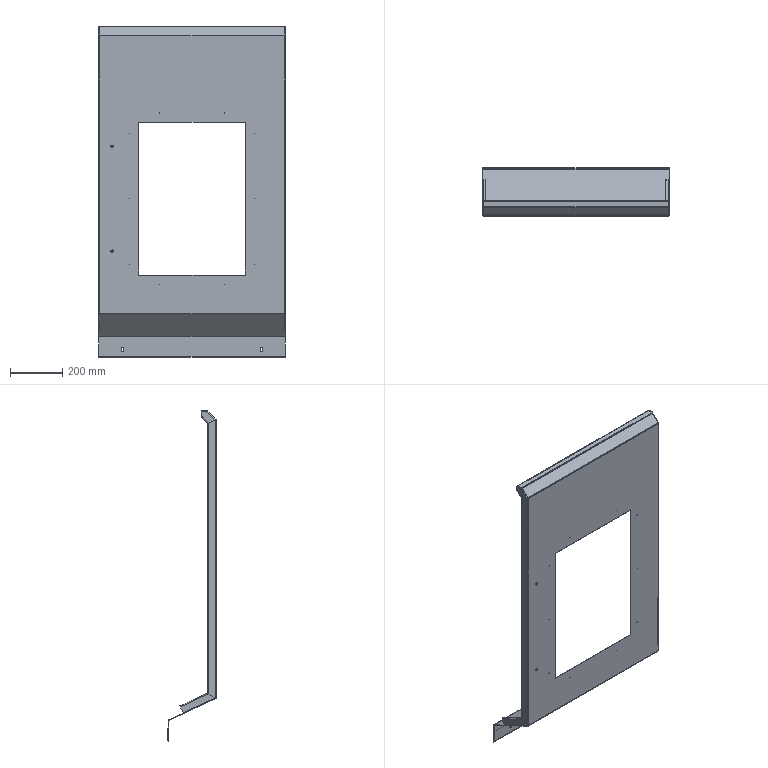Part | NX | features solid 2 | 1 solid | 214 faces | box 710 x 184.004 x 1259 mm | volume 1821069 mm3 | plane 120 | cylinder 80 | spline 14 | commonest cylinder face diameters 8 x23 1 x20 4 x17 7 x12 9 x4 0.004 x2